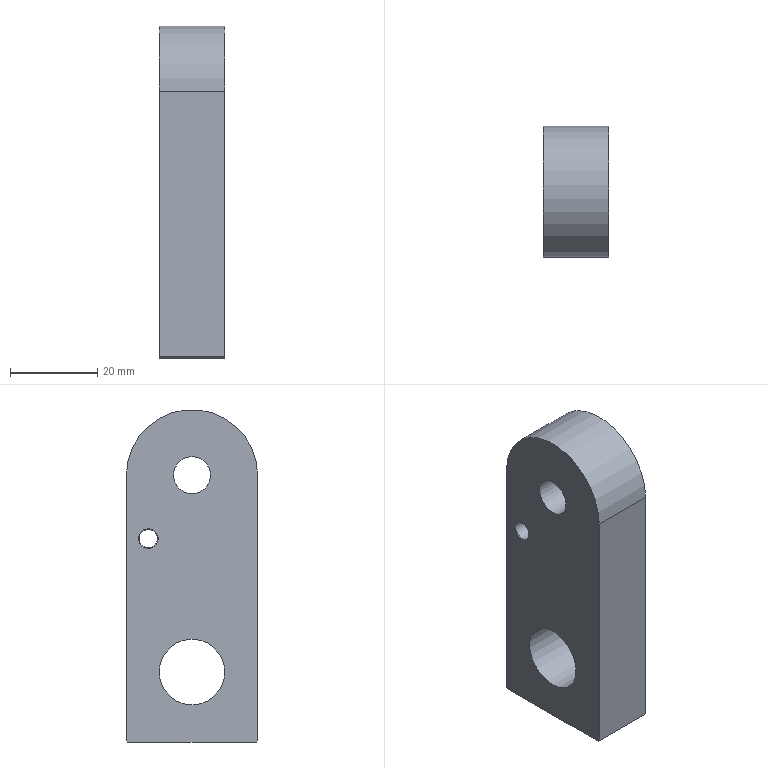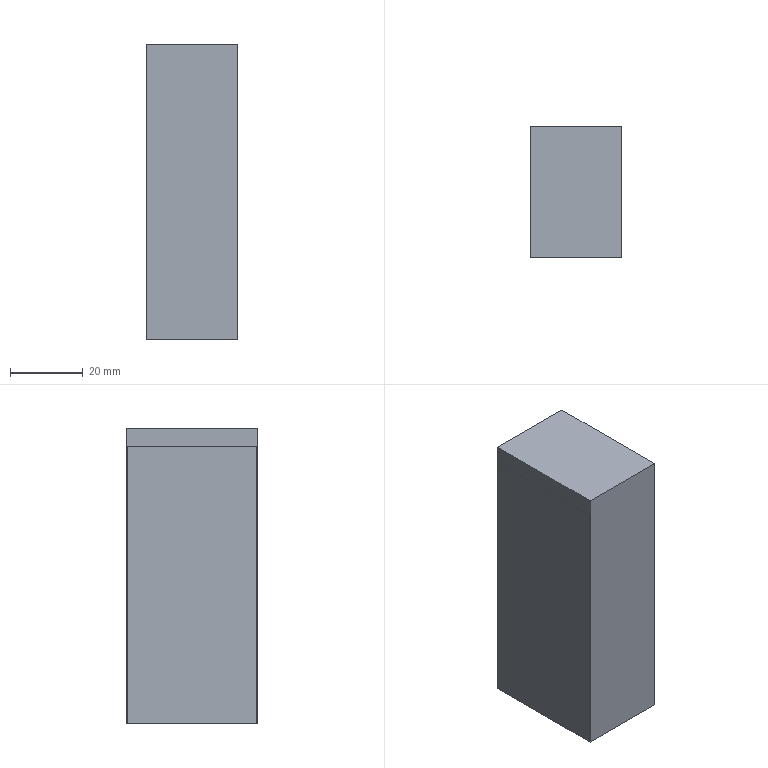CAM job | NX | 3+2 milling, drilling | part box 15 x 30 x 76 mm | stock box 25 x 36 x 81 mm
Tools:
number,name,description,diameter,corner_radius,flute_length,length,flutes
18,D63粗,Milling Tool-5 Parameters,63.0,0.0,50.0,75.0,2
1,D10.粗,Milling Tool-5 Parameters,10.0,0.0,30.0,30.0,4
3,D8点钻,Chamfer Mill,8.0,0.0,50.0,75.0,2
24,D4.,Milling Tool-5 Parameters,4.0,0.0,50.0,75.0,2
18,D63精,Milling Tool-5 Parameters,63.0,0.0,50.0,75.0,2
2,D10精光,Milling Tool-5 Parameters,10.0,0.0,50.0,75.0,2
19,4倒角,Drilling Tool,4.0,0.0,35.0,50.0,2
5,D6.,Milling Tool-5 Parameters,6.0,0.0,50.0,75.0,2
4,Z8.5,Drilling Tool,8.5,0.0,35.0,50.0,2
14,Z4.2,Drilling Tool,4.2,0.0,35.0,50.0,2
15,M5,Drilling Tool,5.0,0.0,35.0,50.0,4
6,D6R0.5,Milling Tool-5 Parameters,6.0,0.5,50.0,75.0,2
20,D5.1钻头,Drilling Tool,5.1,0.0,35.0,50.0,2
21,M6,Drilling Tool,6.0,0.0,35.0,50.0,4
0,D2,Milling Tool-5 Parameters,2.0,0.0,50.0,75.0,2
16,THREAD_MILL,Thread Mill,8.2,0.0,20.0,50.0,20
Operations:
program,operation,operation_type,tool,method,geometry_group,spindle_rpm,surface_speed,feed_per_tooth,feed_cut,feed_plunge,cut_length_mm,path_length_mm,cut_time_min,machine_time_min
G54,FLOOR_FACING_COPY_2_1,VolumeBased25DMillingOperation,D63粗,METHOD,WORKPIECE,1600.0,316.0,0.3125,1000.0,100.0,175.0,268.8,0.175,0.1844
G54,ADAPTIVE_MILLING,CavityMilling,D10.粗,METHOD,WORKPIECE,3200.0,100.0,0.2344,3000.0,100.0,3539.588,3664.588,0.8982,0.9107
G54,DRILLING,Operation,D8点钻,DRILL_METHOD,WORKPIECE,1500.0,37.0,0.0333,100.0,0.0,17.1,217.537,0.171,0.191
G54,PECK_DRILLING,Operation,Z8.5,METHOD,WORKPIECE,1200.0,19.0,0.0333,80.0,0.0,50.0,248.1,0.625,0.6448
G54,PECK_DRILLING_COPY_1,Operation,Z4.2,METHOD,WORKPIECE,1200.0,19.0,0.0333,80.0,0.0,23.0,146.0,0.2875,0.2998
G54,CURVE_DRIVE,SurfaceContour,D6R0.5,METHOD,WORKPIECE,4000.0,75.0,0.1875,1500.0,100.0,490.329,584.995,0.3269,0.3364
G54,PECK_DRILLING_COPY_1_COPY,Operation,M5,METHOD,WORKPIECE,200.0,3.0,0.001,0.8,0.0,11.0,122.0,13.75,13.761
G54,THREAD_MILLING,ThreadMilling,THREAD_MILL,METHOD,WORKPIECE,3000.0,77.0,0.025,150.0,100.0,243.748,579.09,1.625,1.659
G54,HOLE_MILLING_COPY,CylinderMilling,D6.,METHOD,WORKPIECE,2800.0,35.0,0.1429,800.0,100.0,2322.318,2437.818,2.903,2.914
G54,PLANAR_MILL_2,PlanarMilling,D6.,METHOD,WORKPIECE,3000.0,56.0,0.05,300.0,100.0,118.384,245.384,0.3946,0.4073
G54,FLOOR_FACING_COPY_2_1_COPY_COPY,VolumeBased25DMillingOperation,D63精,METHOD,WORKPIECE,1800.0,316.0,0.3125,400.0,100.0,165.0,259.0,0.4125,0.4219
G54,PLANAR_MILL,PlanarMilling,D10精光,METHOD,WORKPIECE,2000.0,75.0,0.1,400.0,100.0,476.783,607.783,1.192,1.205
G54,PLANAR_MILL_COPY,PlanarMilling,4倒角,METHOD,WORKPIECE,5000.0,62.0,0.06,600.0,100.0,214.434,317.434,0.3574,0.3677
G54,PLANAR_MILL_COPY_COPY,PlanarMilling,4倒角,METHOD,WORKPIECE,5000.0,62.0,0.06,600.0,100.0,100.374,203.374,0.1673,0.1776
G54,CURVE_DRIVE_COPY,SurfaceContour,D6R0.5,METHOD,WORKPIECE,4000.0,75.0,0.1875,1500.0,100.0,490.329,584.995,0.3269,0.3364
反面,ADAPTIVE_MILLING_COPY,CavityMilling,D10.粗,METHOD,WORKPIECE_1,3200.0,100.0,0.2344,3000.0,100.0,8908.456,9002.256,2.97,2.979
反面,FLOOR_FACING_COPY_2_1_COPY_COPY_COPY_COPY_COPY,VolumeBased25DMillingOperation,D63精,METHOD,WORKPIECE_1,1800.0,316.0,0.3125,400.0,100.0,165.0,259.0,0.4125,0.4219
反面,DRILLING_COPY,Operation,D8点钻,DRILL_METHOD,WORKPIECE_1,3500.0,87.0,0.0429,300.0,0.0,5.5,71.0,0.0183,0.0249
反面,PLANAR_MILL_COPY_COPY_COPY_2,PlanarMilling,4倒角,METHOD,WORKPIECE_1,4500.0,113.0,0.0889,800.0,100.0,214.11,317.11,0.2676,0.2779
反面,PLANAR_MILL_COPY_COPY_COPY_2_COPY,PlanarMilling,4倒角,METHOD,WORKPIECE_1,4500.0,113.0,0.0889,800.0,100.0,76.719,326.421,0.0959,0.1209
PROGRAM_1,DRILLING_1,Operation,4倒角,METHOD,MCS_1,1600.0,20.0,0.0187,60.0,0.0,4.5,69.0,0.075,0.0814
PROGRAM_1,DRILLING_2,Operation,D5.1钻头,METHOD,MCS_1,1300.0,20.0,0.0231,60.0,0.0,15.0,90.0,0.25,0.2575
PROGRAM_1,HOLE_MILLING,CylinderMilling,D4.,METHOD,MCS_1,3000.0,37.0,0.0833,500.0,100.0,796.452,864.053,1.593,1.6
PROGRAM_1,PLANAR_MILL_1,PlanarMilling,4倒角,METHOD,MCS_1,3000.0,37.0,0.1,600.0,100.0,20.252,78.852,0.0338,0.0396
PROGRAM_1,DRILLING_1_COPY,Operation,4倒角,METHOD,MCS_1,1600.0,20.0,0.0187,60.0,0.0,4.5,112.748,0.075,0.0858
PROGRAM_1,DRILLING_2_COPY,Operation,D5.1钻头,METHOD,MCS_1,1300.0,20.0,0.0231,60.0,0.0,15.0,133.748,0.25,0.2619
PROGRAM_1,DRILLING_2_COPY_COPY,Operation,M6,METHOD,MCS_1,300.0,5.0,0.25,300.0,0.0,13.0,129.748,0.0433,0.055
PROGRAM,PLANAR_PROFILING,PlanarMilling,D2,METHOD,MCS_2,3000.0,18.0,0.1333,800.0,100.0,5755.759,27936.259,7.195,9.413